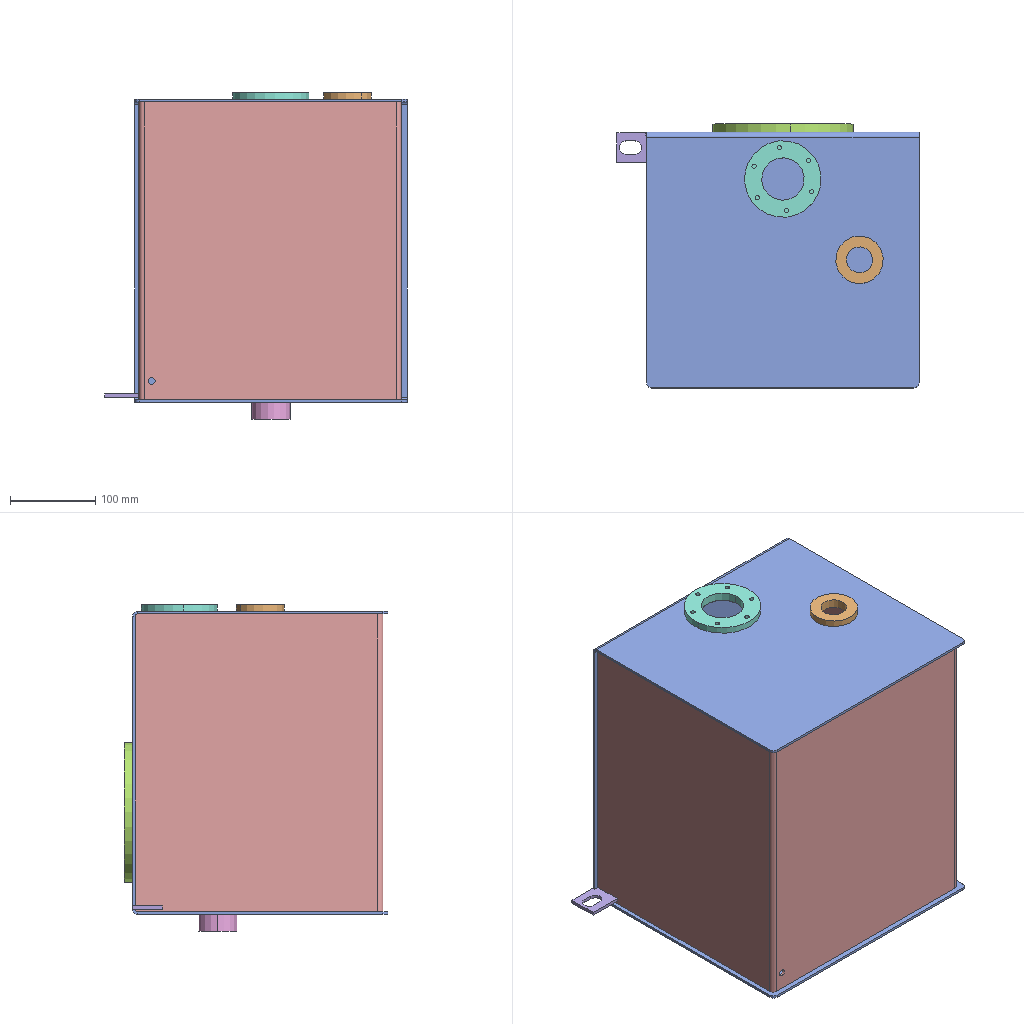Assembly | SolidWorks | 7 different items | 7 placed | box 355 x 310 x 384 mm
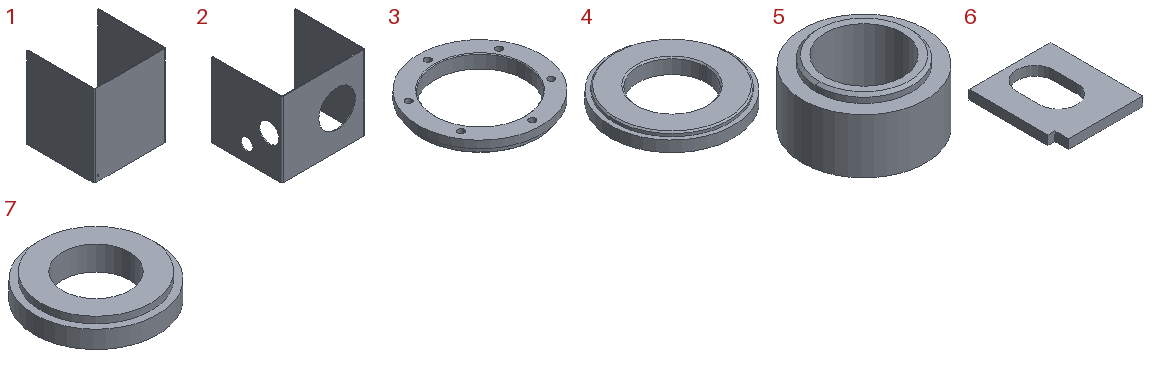Parts list (item | quantity | size | volume | features):
1 | x1 | 308 x 291 x 350 mm | 923970 mm3 | features ICE 2, FlatPattern 1, SMBaseFlange 1, SheetMetal 1
2 | x1 | 356 x 300 x 320 mm | 825456 mm3 | features ICE 4, FlatPattern 1, SMBaseFlange 1, SheetMetal 1
3 | x1 | 165 x 165 x 18 mm | 159935 mm3 | features ICE 2, Chamfer 1, Extrusion 1
4 | x1 | 90 x 90 x 11 mm | 45003 mm3 | features ICE 2, Chamfer 1, Extrusion 1
5 | x1 | 45 x 45 x 23 mm | 20434 mm3 | features Chamfer 1, Extrusion 1, ICE 1
6 | x1 | 35 x 40 x 4 mm | 4084 mm3 | features Extrusion 1
7 | x1 | 56 x 56 x 11 mm | 17612 mm3 | features ICE 2, Extrusion 1
Mates (type | each side: item.copy, entity, surface, feature):
Coincident | 1.1 face plane Base-Flange1 | 2.1 face plane Base-Flange1 | 2 times
DistanceDim | 1.1 face plane Base-Flange1 | 2.1 face plane Base-Flange1
Coincident | 2.1 face plane Base-Flange1 | 3.1 face plane Boss-Extrude1
Concentric | 2.1 edge | 3.1 edge
Coincident | 2.1 face plane Base-Flange1 | 5.1 face plane Boss-Extrude1
Concentric | 2.1 edge | 5.1 edge
Coincident | 2.1 face plane Base-Flange1 | 4.1 face plane Boss-Extrude1
Concentric | 2.1 edge | 4.1 edge
Coincident | 2.1 face plane Base-Flange1 | 7.1 face plane Boss-Extrude1
Concentric | 2.1 edge | 7.1 edge
Coincident | 1.1 face plane Base-Flange1 | 6.1 face plane Boss-Extrude1
DistanceDim | 6.1 face plane Boss-Extrude1 | 2.1 face plane Base-Flange1
Coincident | 2.1 face plane Base-Flange1 | 6.1 face plane Boss-Extrude1